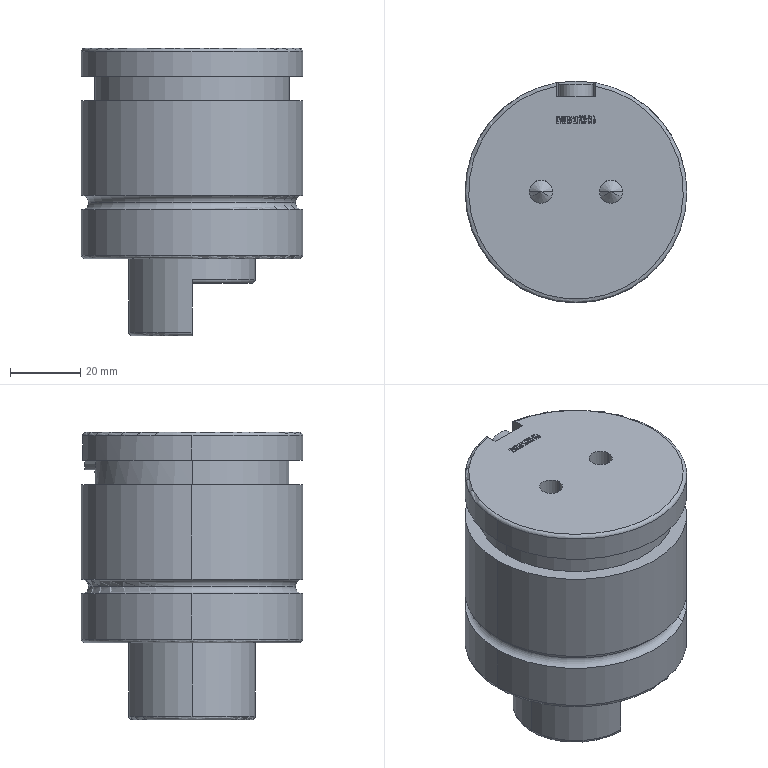Part | STEP file | 1_id406_x_t | 1 solid | 196 faces | box 63.2 x 63.2 x 82 mm | volume 195546 mm3 | plane 135 | cylinder 22 | other 21 | cone 12 | torus 6 | commonest cylinder face diameters 63.2 x7 4.9 x4 6.6 x4 9.5 x2 36 x2 55.6 x2